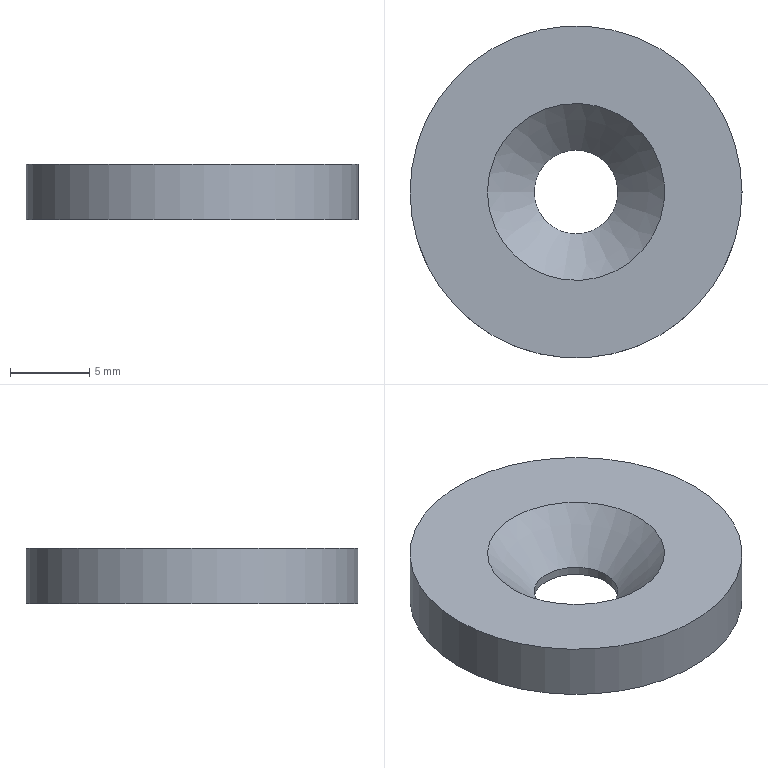Part | NX | 1 solid | 5 faces | box 21 x 21 x 3.5 mm | volume 1036 mm3 | cylinder 2 | plane 2 | cone 1 | commonest cylinder face diameters 5.3 x1 21 x1
STEP:
#1=CARTESIAN_POINT('',(-2.65,0.,0.55));
#2=VERTEX_POINT('',#1);
#3=CARTESIAN_POINT('',(0.,0.,0.55));
#4=DIRECTION('',(0.,0.,-1.));
#5=DIRECTION('',(-1.,0.,0.));
#6=AXIS2_PLACEMENT_3D('',#3,#4,#5);
#7=CIRCLE('',#6,2.65);
#8=EDGE_CURVE('',#2,#2,#7,.T.);
#9=ORIENTED_EDGE('',*,*,#8,.F.);
#10=EDGE_LOOP('',(#9));
#11=FACE_BOUND('',#10,.T.);
#12=CARTESIAN_POINT('',(-2.65,0.,0.));
#13=VERTEX_POINT('',#12);
#14=CARTESIAN_POINT('',(0.,0.,0.));
#15=DIRECTION('',(0.,0.,-1.));
#16=DIRECTION('',(-1.,0.,0.));
#17=AXIS2_PLACEMENT_3D('',#14,#15,#16);
#18=CIRCLE('',#17,2.65);
#19=EDGE_CURVE('',#13,#13,#18,.T.);
#20=ORIENTED_EDGE('',*,*,#19,.T.);
#21=EDGE_LOOP('',(#20));
#22=FACE_BOUND('',#21,.T.);
#23=CARTESIAN_POINT('',(0.,0.,0.));
#24=DIRECTION('',(0.,0.,-1.));
#25=DIRECTION('',(1.,0.,0.));
#26=AXIS2_PLACEMENT_3D('',#23,#24,#25);
#27=CYLINDRICAL_SURFACE('',#26,2.65);
#28=ADVANCED_FACE('',(#11,#22),#27,.F.);
#29=CARTESIAN_POINT('',(-5.6,0.,3.5));
#30=VERTEX_POINT('',#29);
#31=CARTESIAN_POINT('',(0.,0.,3.5));
#32=DIRECTION('',(0.,0.,-1.));
#33=DIRECTION('',(-1.,0.,0.));
#34=AXIS2_PLACEMENT_3D('',#31,#32,#33);
#35=CIRCLE('',#34,5.6);
#36=EDGE_CURVE('',#30,#30,#35,.T.);
#37=ORIENTED_EDGE('',*,*,#36,.F.);
#38=EDGE_LOOP('',(#37));
#39=FACE_BOUND('',#38,.T.);
#40=ORIENTED_EDGE('',*,*,#8,.T.);
#41=EDGE_LOOP('',(#40));
#42=FACE_BOUND('',#41,.T.);
#43=CARTESIAN_POINT('',(0.,0.,0.55));
#44=DIRECTION('',(0.,0.,1.));
#45=DIRECTION('',(-1.,0.,0.));
#46=AXIS2_PLACEMENT_3D('',#43,#44,#45);
#47=CONICAL_SURFACE('',#46,2.65,45.);
#48=ADVANCED_FACE('',(#39,#42),#47,.F.);
#49=CARTESIAN_POINT('',(-10.5,0.,3.5));
#50=VERTEX_POINT('',#49);
#51=CARTESIAN_POINT('',(0.,0.,3.5));
#52=DIRECTION('',(0.,0.,-1.));
#53=DIRECTION('',(-1.,0.,0.));
#54=AXIS2_PLACEMENT_3D('',#51,#52,#53);
#55=CIRCLE('',#54,10.5);
#56=EDGE_CURVE('',#50,#50,#55,.T.);
#57=ORIENTED_EDGE('',*,*,#56,.F.);
#58=EDGE_LOOP('',(#57));
#59=FACE_BOUND('',#58,.T.);
#60=ORIENTED_EDGE('',*,*,#36,.T.);
#61=EDGE_LOOP('',(#60));
#62=FACE_BOUND('',#61,.T.);
#63=CARTESIAN_POINT('',(0.,5.6,3.5));
#64=DIRECTION('',(0.,0.,-1.));
#65=DIRECTION('',(1.,0.,0.));
#66=AXIS2_PLACEMENT_3D('',#63,#64,#65);
#67=PLANE('',#66);
#68=ADVANCED_FACE('',(#59,#62),#67,.F.);
#69=CARTESIAN_POINT('',(-10.5,0.,0.));
#70=VERTEX_POINT('',#69);
#71=CARTESIAN_POINT('',(0.,0.,0.));
#72=DIRECTION('',(0.,0.,-1.));
#73=DIRECTION('',(-1.,0.,0.));
#74=AXIS2_PLACEMENT_3D('',#71,#72,#73);
#75=CIRCLE('',#74,10.5);
#76=EDGE_CURVE('',#70,#70,#75,.T.);
#77=ORIENTED_EDGE('',*,*,#76,.F.);
#78=EDGE_LOOP('',(#77));
#79=FACE_BOUND('',#78,.T.);
#80=ORIENTED_EDGE('',*,*,#56,.T.);
#81=EDGE_LOOP('',(#80));
#82=FACE_BOUND('',#81,.T.);
#83=CARTESIAN_POINT('',(0.,0.,0.));
#84=DIRECTION('',(0.,0.,-1.));
#85=DIRECTION('',(1.,0.,0.));
#86=AXIS2_PLACEMENT_3D('',#83,#84,#85);
#87=CYLINDRICAL_SURFACE('',#86,10.5);
#88=ADVANCED_FACE('',(#79,#82),#87,.T.);
#89=ORIENTED_EDGE('',*,*,#19,.F.);
#90=EDGE_LOOP('',(#89));
#91=FACE_BOUND('',#90,.T.);
#92=ORIENTED_EDGE('',*,*,#76,.T.);
#93=EDGE_LOOP('',(#92));
#94=FACE_BOUND('',#93,.T.);
#95=CARTESIAN_POINT('',(0.,10.5,0.));
#96=DIRECTION('',(0.,0.,1.));
#97=DIRECTION('',(-1.,0.,0.));
#98=AXIS2_PLACEMENT_3D('',#95,#96,#97);
#99=PLANE('',#98);
#100=ADVANCED_FACE('',(#91,#94),#99,.F.);
#101=CLOSED_SHELL('',(#28,#48,#68,#88,#100));
#102=MANIFOLD_SOLID_BREP('',#101);
#103=(LENGTH_UNIT()NAMED_UNIT(*)SI_UNIT(.MILLI.,.METRE.));
#104=UNCERTAINTY_MEASURE_WITH_UNIT(LENGTH_MEASURE(0.00002),#103,'','');
#105=(NAMED_UNIT(*)PLANE_ANGLE_UNIT()SI_UNIT($,.RADIAN.));
#106=PLANE_ANGLE_MEASURE_WITH_UNIT(PLANE_ANGLE_MEASURE(0.01745),#105);
#107=DIMENSIONAL_EXPONENTS(0.,0.,0.,0.,0.,0.,0.);
#108=(CONVERSION_BASED_UNIT('DEGREE',#106)NAMED_UNIT(#107)PLANE_ANGLE_UNIT());
#109=(NAMED_UNIT(*)SI_UNIT($,.STERADIAN.)SOLID_ANGLE_UNIT());
#110=(GEOMETRIC_REPRESENTATION_CONTEXT(3)GLOBAL_UNCERTAINTY_ASSIGNED_CONTEXT((#104))GLOBAL_UNIT_ASSIGNED_CONTEXT((#103,#108,#109))REPRESENTATION_CONTEXT('',''));
#111=ADVANCED_BREP_SHAPE_REPRESENTATION('',(#102),#110);